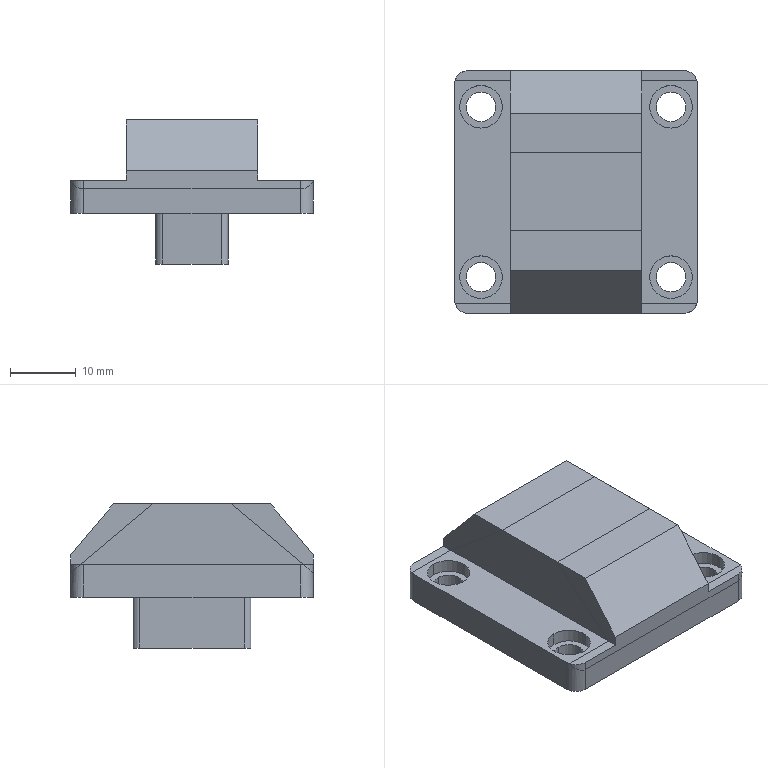NC program | NX | posted by the shop | part box 37 x 37 x 22 mm
Whole program:
G40 G17 G49 G80 G90 G54
M05
M09
G91 G28 Z0.0
M01
T13 M06
S4500 M03
G00 G90 G54 X-55.5 Y0.0
T02
G43 Z20. H13 M08
Z6.025
G01 Z3.025 F1200.
X-30.5
X30.5
X55.5
Z6.025
G00 Z20.
X-55.5
Z5.05
G01 Z2.05
X-30.5
X30.5
X55.5
Z5.05
G00 Z20.
X-55.5
Z4.075
G01 Z1.075
X-30.5
X30.5
X55.5
Z4.075
G00 Z20.
X-55.5
Z3.1
G01 Z.1
X-30.5
X30.5
X55.5
Z3.1
G00 Z20.
G00 X-55.5 Y0.0 S4500 M03
Z3.
G01 Z0.0 F800.
X-30.5
X30.5
X55.5
Z3.
G00 Z20.
M05
M09
G91 G28 Z0.0
M01
T02 M06
S5500 M03
G00 G90 G54 X-27.497 Y-1.157
T03
G43 Z20. H02 M08
Z-4.65
G01 Z-7.65 F2500.
X-25.918 Y-.369
G03 X-25.579 Y-.05 I-.396 J.76
X-24.949 Y2.444 I-5.577 J2.735
X-24.707 Y10.282 I-90.433 J6.724
G02 X-24.668 Y19.672 I350.603 J3.267
X-22.035 Y23.129 I4.845 J-.96
X-17.147 Y24.45 I5.608 J-11.042
X-8.553 Y24.695 I7.203 J-101.747
G01 X-3.753 Y24.7
X19.321 Y24.697
G02 X22.892 Y22.42 I-.428 J-4.61
X24.401 Y17.596 I-9.561 J-5.639
X24.695 Y8.605 I-88.325 J-7.39
G01 X24.7 Y3.905
X24.697 Y-19.321
G02 X22.42 Y-22.892 I-4.608 J.427
X17.596 Y-24.401 I-5.646 J9.582
X8.605 Y-24.695 I-7.39 J88.285
G01 X3.905 Y-24.7
X-19.321 Y-24.697
G02 X-22.892 Y-22.42 I.427 J4.608
X-24.401 Y-17.596 I9.581 J5.645
X-24.695 Y-8.605 I88.287 J7.39
X-24.64 Y-1.807 I113.874 J2.474
G03 X-23.912 Y11.088 I-93.764 J11.765
G02 X-23.87 Y17.373 I572.333 J-.604
X-20.54 Y22.08 I6.134 J-.808
X-14.982 Y23.607 I6.481 J-12.713
X-4.89 Y23.896 I8.248 J-111.568
G01 X-.49 Y23.899
X16.873
G02 X21.928 Y20.798 I-.222 J-6.031
X23.586 Y15.179 I-11.855 J-6.552
X23.896 Y4.988 I-105.927 J-8.328
G01 X23.899 Y.588
Y-16.873
G02 X20.797 Y-21.928 I-6.031 J.222
X15.179 Y-23.585 I-6.556 J11.871
X4.988 Y-23.896 I-8.333 J105.935
G01 X.588 Y-23.899
X-16.873
G02 X-21.928 Y-20.797 I.222 J6.031
X-23.585 Y-15.179 I11.871 J6.556
X-23.779 Y-2.092 I98.638 J8.005
G03 X-23.1 Y14.877 I-160.957 J14.935
G02 X-19.171 Y21.185 I7.066 J-.024
X-13.211 Y22.786 I7.006 J-14.193
X-2.42 Y23.096 I8.799 J-118.165
G01 X1.98 Y23.099
G02 X15.48 Y23.069 I4.982 J-797.107
X21.185 Y19.171 I-.621 J-7.033
X22.786 Y13.209 I-14.196 J-7.009
X23.096 Y2.317 I-120.55 J-8.883
G01 X23.099 Y-2.083
G02 X23.069 Y-15.482 I-790.217 J-4.913
X19.17 Y-21.185 I-7.031 J.623
X13.211 Y-22.785 I-7.004 J14.183
X2.92 Y-23.095 I-8.54 J112.616
G01 X-1.48 Y-23.099
G02 X-15.48 Y-23.069 I-5.249 J819.414
X-21.184 Y-19.17 I.621 J7.032
X-22.785 Y-13.211 I14.18 J7.004
X-22.678 Y1.393 I81.617 J6.705
G03 X-22.287 Y13.696 I-225.961 J13.343
G02 X-17.748 Y20.414 I7.795 J-.374
X-11.281 Y22.008 I7.478 J-16.415
X-.688 Y22.295 I8.854 J-131.204
X13.811 Y22.267 I5.684 J-799.484
X20.37 Y17.828 I-.454 J-7.736
X21.99 Y11.47 I-15.899 J-7.438
X22.294 Y1.378 I-118.327 J-8.608
X22.266 Y-13.821 I-834.287 J-6.101
X17.893 Y-20.336 I-7.722 J.459
X11.643 Y-21.972 I-7.395 J15.489
X.852 Y-22.295 I-8.954 J118.83
X-13.848 Y-22.264 I-5.694 J800.086
X-20.397 Y-17.77 I.503 J7.752
X-21.986 Y-11.501 I15.991 J7.39
X-22.029 Y-1.013 I64.152 J5.506
G03 X-21.493 Y12.316 I-282.44 J18.029
G02 X-16.507 Y19.601 I8.369 J-.379
X-9.929 Y21.191 I7.733 J-17.589
X1.263 Y21.495 I9.297 J-136.127
X12.363 Y21.46 I3.956 J-503.291
X19.595 Y16.515 I-.375 J-8.31
X21.19 Y9.934 I-17.546 J-7.736
X21.494 Y-.858 I-130.568 J-9.083
X21.46 Y-12.357 I-561.05 J-4.083
X16.515 Y-19.594 I-8.308 J.369
X9.934 Y-21.189 I-7.737 J17.55
X-.858 Y-21.494 I-9.078 J130.164
X-12.357 Y-21.46 I-4.088 J558.524
X-19.593 Y-16.515 I.372 J8.311
X-21.188 Y-9.935 I17.482 J7.721
X-21.17 Y-.344 I64.835 J4.68
G03 X-20.707 Y11.039 I-478.167 J25.18
G02 X-15.279 Y18.82 I8.869 J-.403
X-8.586 Y20.385 I7.922 J-18.791
X2.906 Y20.695 I9.556 J-140.96
X11.305 Y20.634 I2.943 J-172.632
X18.774 Y15.361 I-.58 J-8.747
X20.384 Y8.585 I-18.495 J-7.974
X20.693 Y-2.007 I-129.859 J-9.089
X20.634 Y-11.305 I-198.613 J-3.382
X15.36 Y-18.773 I-8.743 J.579
X8.584 Y-20.383 I-7.978 J18.509
X-2.708 Y-20.694 I-9.452 J137.955
X-11.307 Y-20.633 I-3.051 J175.551
X-18.772 Y-15.361 I.582 J8.745
X-20.394 Y-8.184 I18.412 J7.933
X-20.325 Y.21 I73.859 J3.592
G01 X-19.924 Y9.858
G02 X-14.196 Y17.997 I9.266 J-.436
X-7.308 Y19.58 I8.169 J-19.764
X4.184 Y19.894 I9.646 J-142.751
X10.481 Y19.787 I1.925 J-71.699
X17.907 Y14.366 I-.913 J-9.048
X19.57 Y7.399 I-19.01 J-8.222
X19.893 Y-3.593 I-132.685 J-9.389
X19.796 Y-10.39 I-85.947 J-2.178
X14.365 Y-17.906 I-9.056 J.823
X7.398 Y-19.57 I-8.231 J19.053
X-4.094 Y-19.894 I-9.652 J138.449
X-10.491 Y-19.785 I-1.972 J72.106
X-17.905 Y-14.365 I.925 J9.047
X-19.535 Y-7.09 I18.206 J7.899
X-19.394 Y2.902 I100.414 J3.577
X-19.076 Y9.369 I102.995 J-1.822
X-13.318 Y17.103 I9.484 J-1.05
X-6.246 Y18.762 I8.411 J-19.941
X8.745 Y19.03 I10.15 J-148.446
X17.144 Y13.191 I-.355 J-9.471
X18.783 Y6.003 I-20.401 J-8.432
X19.027 Y-8.788 I-151.705 J-9.903
X13.297 Y-17.094 I-9.439 J.382
X6.223 Y-18.762 I-8.411 J19.835
X-8.768 Y-19.028 I-10.115 J147.225
X-17.119 Y-13.235 I.365 J9.442
X-18.681 Y-5.839 I18.859 J7.845
X-18.524 Y4.683 I127.369 J3.363
X-17.991 Y9.843 I22.958 J.239
X-12.291 Y16.293 I9.484 J-2.638
X-5.21 Y17.947 I8.531 J-20.54
X7.879 Y18.199 I8.613 J-107.126
X16.273 Y12.286 I-.539 J-9.681
X17.944 Y5.215 I-20.255 J-8.519
X18.2 Y-7.874 I-106.842 J-8.634
X12.286 Y-16.272 I-9.682 J.537
X5.009 Y-17.962 I-8.615 J20.581
X-7.88 Y-18.199 I-8.41 J106.644
X-16.304 Y-12.183 I.53 J9.648
X-17.816 Y-4.774 I19.397 J7.817
X-17.534 Y7.115 I99.994 J3.573
X-11.243 Y15.507 I10.092 J-1.012
X-3.861 Y17.166 I8.758 J-21.716
X6.829 Y17.382 I7.011 J-82.036
X15.462 Y11.278 I-.536 J-9.915
X17.139 Y4.103 I-20.789 J-8.644
X17.377 Y-6.885 I-79.989 J-7.231
X11.269 Y-15.464 I-9.91 J.592
X3.889 Y-17.158 I-8.753 J21.218
X-6.9 Y-17.376 I-7.002 J79.46
X-15.456 Y-11.217 I.572 J9.818
X-16.946 Y-3.904 I19.638 J7.809
X-16.738 Y6.185 I70.453 J3.598
X-10.354 Y14.661 I10.284 J-1.105
X-2.972 Y16.345 I8.856 J-21.802
X6.017 Y16.538 I5.754 J-58.453
X14.611 Y10.379 I-.705 J-10.06
X16.317 Y3.213 I-20.803 J-8.737
X16.533 Y-6.075 I-57.63 J-5.987
X10.498 Y-14.554 I-10.013 J.739
X3.141 Y-16.322 I-8.869 J20.711
X-6.146 Y-16.525 I-5.877 J56.36
X-14.661 Y-10.137 I.802 J9.939
X-16.087 Y-2.913 I20.411 J7.781
X-15.89 Y5.573 I47.341 J3.148
X-9.478 Y13.819 I10.379 J-1.456
X-2.097 Y15.525 I8.948 J-21.889
X5.589 Y15.638 I4.412 J-38.619
X13.73 Y9.564 I-1.187 J-10.083
X15.508 Y2.211 I-20.822 J-8.925
X15.663 Y-5.376 I-40.157 J-4.619
X9.562 Y-13.729 I-10.103 J.975
X2.105 Y-15.517 I-8.985 J21.029
X-5.581 Y-15.638 I-4.447 J38.207
X-13.711 Y-9.429 I1.123 J9.898
X-15.221 Y-2.118 I20.105 J7.962
X-15.004 Y5.063 I32.126 J2.627
X-8.727 Y12.925 I10.383 J-1.853
X-1.271 Y14.702 I9.071 J-21.524
X5.31 Y14.682 I3.214 J-25.35
X12.842 Y8.772 I-1.788 J-10.034
X14.667 Y1.534 I-20.213 J-8.944
X14.709 Y-5.148 I-26.482 J-3.508
X8.703 Y-12.875 I-10.073 J1.632
X1.258 Y-14.694 I-9.054 J20.903
X-5.323 Y-14.679 I-3.231 J25.084
X-12.842 Y-8.539 I1.76 J9.828
X-14.372 Y-1.033 I20.434 J8.077
X-13.928 Y5.224 I19.945 J1.727
X-7.881 Y12.081 I10.208 J-2.908
X-5.543 Y13.05 I8.337 J-16.801
X3.777 Y13.896 I7.185 J-27.408
X11.957 Y7.985 I-1.097 J-10.135
X13.86 Y.463 I-19.902 J-9.035
X13.506 Y-5.689 I-16.244 J-2.152
X7.807 Y-12.04 I-9.841 J3.099
G03 X7.075 Y-12.46 I1.236 J-3.
G02 X3.586 Y-13.464 I-5.023 J10.888
X-3.977 Y-13.868 I-5.169 J25.796
X-11.909 Y-7.794 I1.263 J9.865
X-13.502 Y.705 I19.712 J8.093
X-11.821 Y7.198 I11.771 J.416
X-9.247 Y9.968 I10.356 J-7.04
X-8.142 Y11.642 I5.783 J-2.617
G01 X-7.075 Y12.46
X-5.833 Y12.975
X-4.498 Y13.15
X4.502
X5.833 Y12.975
X7.075 Y12.46
G02 X9.71 Y9.759 I-5.546 J-8.045
X12.786 Y1.583 I-15.282 J-10.417
X12.618 Y-4.767 I-15.018 J-2.78
X9.341 Y-9.722 I-9.822 J2.934
G01 X8.96 Y-10.575
X8.142 Y-11.642
X7.269 Y-12.311
G03 X8.12 Y-13.659 I.487 J-.635
G01 X9.546 Y-12.999 Z-7.55
X10.085 Y-12.754
X10.616 Y-12.492
X10.805 Y-12.311
X12.135 Y-10.546
X13.448 Y-8.769
G03 X14.998 Y-5.194 I-8.345 J5.741
X15.395 Y-1.566 I-13.07 J3.268
X14.975 Y2.967 I-23.56 J.104
X14.082 Y6.365 I-30.493 J-6.204
X13.047 Y8.86 I-20.441 J-7.013
G01 X12.341 Y10.306
X11.617 Y11.744
G03 X11.248 Y12.035 I-.68 J-.485
G01 X9.959 Y12.531
X8.946 Y12.91 Z-7.619
X8.699 Y12.973 Z-7.634
X8.467 Y12.866 Z-7.65
G03 X8.142 Y11.642 I.31 J-.738
G01 X8.96 Y10.575
G02 X11.338 Y4.09 I-45.173 J-20.246
X11.928 Y-2.741 I-17.08 J-4.917
X9.799 Y-7.623 I-10.739 J1.777
G01 X9.65 Y-8.002
X9.475 Y-9.333
X9.245 Y-9.887
G03 X10.629 Y-10.667 I.739 J-.306
G01 X11.447 Y-9.326 Z-7.55
X11.87 Y-8.607
X11.925 Y-8.34
X12.463 Y8.532
G03 X12.09 Y9.234 I-.803 J.024
G01 X11.433 Y9.649
X10.591 Y10.169 Z-7.613
X10.414 Y10.273 Z-7.625
X10.21 Y10.283 Z-7.638
X10.023 Y10.199 Z-7.65
G03 X9.475 Y9.333 I.246 J-.762
X10.502 Y4.124 I41.513 J5.479
G02 X10.948 Y-2.026 I-16.845 J-4.314
X9.685 Y-5.868 I-15.115 J2.841
G03 X9.65 Y-8.002 I19.386 J-1.388
X10.521 Y-8.798 I.8 J0.0
G01 X10.811 Y-8.766 Z-7.632
X11.054 Y-8.599 Z-7.614
X11.189 Y-8.34 Z-7.596
X11.606 Y-7.743 Z-7.55
X12.247 Y-6.807
X12.305 Y-6.635
X12.33 Y-6.454
Y6.451
G03 X12.186 Y6.909 I-.832 J-.01
G01 X11.625 Y7.712
X11.021 Y8.558 Z-7.616
X10.829 Y8.757 Z-7.633
X10.555 Y8.791 Z-7.65
G03 X9.65 Y7.998 I-.104 J-.794
X10.009 Y2.591 I31.793 J-.603
G02 X9.65 Y-2.975 I-14.408 J-1.864
G01 Y-6.075
G03 X11.206 Y-6.337 I.8 J0.0
G01 X11.609 Y-4.818 Z-7.55
X11.735 Y-4.356
X11.838 Y-3.887
X12.33 Y4.651
G03 X12.18 Y5.165 I-.819 J.04
G01 X11.629 Y5.93
X11.013 Y6.767 Z-7.616
X10.817 Y6.962 Z-7.633
X10.542 Y6.993 Z-7.65
G03 X9.65 Y6.198 I-.092 J-.795
G01 Y-8.002
X9.475 Y-9.333
X8.96 Y-10.575
X8.142 Y-11.642
X7.075 Y-12.46
X5.833 Y-12.975
X4.498 Y-13.15
X-4.502
X-5.833 Y-12.975
X-7.075 Y-12.46
G02 X-9.406 Y-10.087 I4.531 J6.781
X-12.437 Y-1.598 I14.212 J9.859
X-11.705 Y4.892 I13.08 J1.812
X-9.691 Y8.095 I13.351 J-6.16
G03 X-9.475 Y9.333 I-5.08 J1.527
G01 X-9.13 Y10.164
G03 X-9.762 Y11.263 I-.739 J.306
G01 X-10.035 Y11.299 Z-7.633
X-10.296 Y11.206 Z-7.616
X-10.484 Y11.005 Z-7.6
X-11.098 Y10.526 Z-7.55
X-12.372 Y9.522
X-12.469 Y9.392
X-12.546 Y9.249
X-14.52 Y4.049
X-14.775 Y3.274
X-15.001 Y2.489
G03 X-15.114 Y.88 I5.273 J-1.18
G01 X-14.983 Y-.75
X-14.807 Y-2.376
G03 X-12.988 Y-8.624 I24.561 J3.762
G01 X-11.678 Y-11.642
G03 X-11.223 Y-12.073 I.742 J.327
G01 X-9.94 Y-12.55
X-8.934 Y-12.913 Z-7.618
X-8.679 Y-12.971 Z-7.634
X-8.444 Y-12.856 Z-7.65
G03 X-8.142 Y-11.642 I-.333 J.728
G01 X-8.96 Y-10.575
G02 X-11.344 Y-2.746 I32.624 J14.21
X-10.871 Y3.862 I12.729 J2.411
X-9.672 Y6.46 I86.07 J-38.16
X-9.598 Y8.398 I20.123 J.2
G03 X-10.592 Y9.277 I-.793 J.104
G01 X-10.843 Y9.217 Z-7.634
X-11.041 Y9.051 Z-7.619
X-11.143 Y8.814 Z-7.603
X-11.598 Y8.119 Z-7.55
X-12.202 Y7.18
X-12.253 Y7.019
X-12.277 Y6.851
X-12.463 Y-8.532
G03 X-12.095 Y-9.215 I.804 J-.008
G01 X-11.429 Y-9.643
X-10.596 Y-10.167 Z-7.613
X-10.418 Y-10.272 Z-7.625
X-10.212 Y-10.284 Z-7.638
X-10.023 Y-10.199 Z-7.65
G03 X-9.475 Y-9.333 I-.246 J.762
X-10.39 Y-3.383 I-104.851 J-13.091
G02 X-9.654 Y4.092 I14.358 J2.36
G01 X-9.65 Y6.622
G03 X-11.204 Y6.889 I-.8 J0.0
G01 X-11.609 Y5.37 Z-7.55
X-11.738 Y4.906
X-11.838 Y4.434
X-12.33 Y-6.453
G03 X-12.181 Y-6.954 I.822 J-.029
G01 X-11.629 Y-7.726
X-11.015 Y-8.566 Z-7.616
X-10.821 Y-8.763 Z-7.633
X-10.546 Y-8.794 Z-7.65
G03 X-9.65 Y-8. I.096 J.795
X-9.716 Y-1.449 I-508.24 J-1.883
X-9.65 Y4.176 I-77.085 J3.726
X-10.998 Y4.759 I-.8 J0.0
G01 X-11.215 Y4.539 Z-7.631
X-11.278 Y4.237 Z-7.612
X-11.608 Y3.323 Z-7.55
X-11.884 Y2.572
X-12.139 Y1.813
X-12.15 Y1.676
X-12.151 Y-2.199
X-12.103 Y-2.471
X-11.622 Y-3.806
X-11.158 Y-5.073 Z-7.636
X-11.029 Y-5.252 Z-7.65
G03 X-9.65 Y-4.7 I.579 J.552
G01 Y-.4
G03 X-10.346 Y.4 I-.809 J-.001
G01 X-11.615 Y.577
Z-4.65
G00 Z20.
M05
M09
G91 G28 Z0.0
M01
T03 M06
S4500 M03
G00 G90 G54 X26.5 Y0.0
T04
G43 Z20. H03 M08
Z-4.75
G01 Z-7.75 F800.
X22.2
Y-16.5
G02 X16.5 Y-22.2 I-5.7 J0.0
G01 X-16.5
G02 X-22.2 Y-16.5 I0.0 J5.7
G01 Y16.5
G02 X-16.5 Y22.2 I5.7 J0.0
G01 X16.5
G02 X22.2 Y16.5 I0.0 J-5.7
G01 Y0.0
X17.
Y-16.5
G02 X16.5 Y-17. I-.5 J0.0
G01 X-16.5
G02 X-17. Y-16.5 I0.0 J.5
G01 Y16.5
G02 X-16.5 Y17. I.5 J0.0
G01 X-9.195
Y11.8
G03 X-10.54 Y8. I4.695 J-3.8
G01 Y-8.
G03 X-9.195 Y-11.8 I6.04 J0.0
G01 X-11.8
Y11.8
X-9.195
Y17.
X16.5
G02 X17. Y16.5 I0.0 J-.5
G01 Y0.0
X11.8
Y-11.8
X9.195
G03 X10.54 Y-8. I-4.695 J3.8
G01 Y8.
G03 X9.195 Y11.8 I-6.04 J0.0
G01 X8.386 Y11.146
G02 X9.5 Y8. I-3.886 J-3.146
G01 Y-8.
G02 X4.5 Y-13. I-5. J0.0
G01 X-4.5
G02 X-9.5 Y-8. I0.0 J5.
G01 Y8.
G02 X-4.5 Y13. I5. J0.0
G01 X4.5
G02 X8.386 Y11.146 I0.0 J-5.
G01 X9.195 Y11.8
X11.8
Y0.0
X26.5
Z-4.75
G00 Z20.
M05
M09
G91 G28 Z0.0
M01
T04 M06
S3500 M03
G00 G90 G54 X3.5 Y12.5
T13
G43 Z20. H04 M08
Z1.5
G01 Z-1.5 F800.
Y11.5
G03 X4.5 Y10.5 I1. J0.0
G02 X7. Y8. I0.0 J-2.5
G01 Y-8.
G02 X4.5 Y-10.5 I-2.5 J0.0
G01 X-4.5
G02 X-7. Y-8. I0.0 J2.5
G01 Y8.
G02 X-4.5 Y10.5 I2.5 J0.0
G01 X4.5
G03 X5.5 Y11.5 I0.0 J1.
G01 Y12.387
Z1.5
G00 Z20.
G00 X-21.908 Y-17.5 S3500 M03
Z-6.25
G01 Z-9.25 F800.
X-21.
G03 X-20. Y-16.5 I0.0 J1.
G01 Y16.5
G02 X-16.5 Y20. I3.5 J0.0
G01 X16.5
G02 X20. Y16.5 I0.0 J-3.5
G01 Y-16.5
G02 X16.5 Y-20. I-3.5 J0.0
G01 X-16.5
G02 X-20. Y-16.5 I0.0 J3.5
G03 X-21. Y-15.5 I-1. J0.0
G01 X-22.
Z-6.25
G00 Z20.
M05
M09
G91 G28 Z0.0
G28 Y0.0
M30